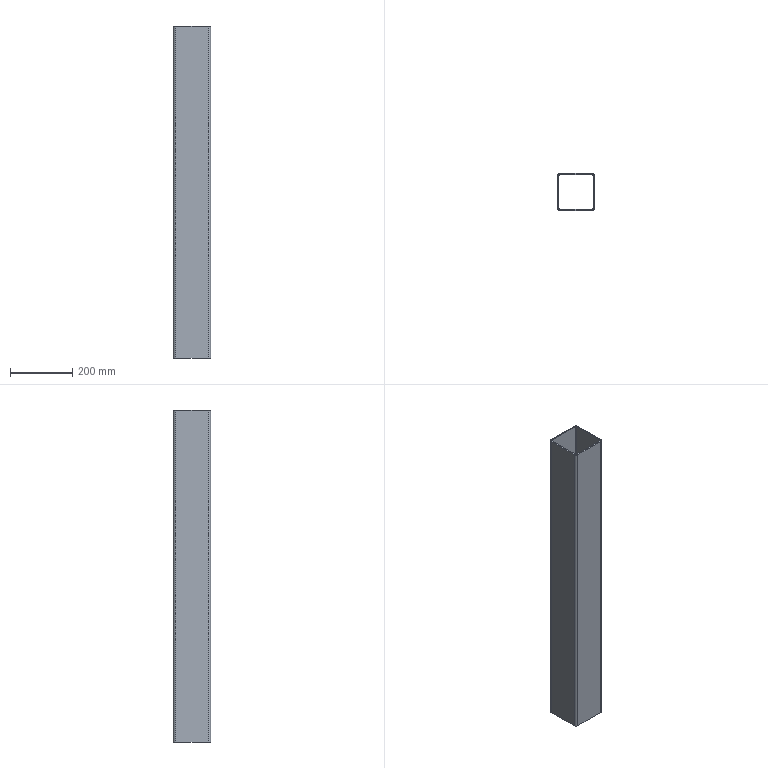Part | SolidWorks | features ICE 1, LibraryFeature 1 | 1 solid | 18 faces | box 120 x 120 x 1070 mm | volume 1941832 mm3 | plane 10 | cylinder 8 | commonest cylinder face diameters 8 x4 16 x4
STEP:
#1=CARTESIAN_POINT('',(52.,60.,-535.));
#2=VERTEX_POINT('',#1);
#3=CARTESIAN_POINT('',(-52.,60.,-535.));
#4=VERTEX_POINT('',#3);
#5=CARTESIAN_POINT('',(0.,60.,-535.));
#6=DIRECTION('',(-1.,0.,0.));
#7=VECTOR('',#6,1000.);
#8=LINE('',#5,#7);
#9=EDGE_CURVE('',#2,#4,#8,.T.);
#10=ORIENTED_EDGE('',*,*,#9,.T.);
#11=CARTESIAN_POINT('',(-52.,60.,535.));
#12=VERTEX_POINT('',#11);
#13=CARTESIAN_POINT('',(-52.,60.,535.));
#14=DIRECTION('',(0.,0.,-1.));
#15=VECTOR('',#14,1000.);
#16=LINE('',#13,#15);
#17=EDGE_CURVE('',#12,#4,#16,.T.);
#18=ORIENTED_EDGE('',*,*,#17,.F.);
#19=CARTESIAN_POINT('',(52.,60.,535.));
#20=VERTEX_POINT('',#19);
#21=CARTESIAN_POINT('',(0.,60.,535.));
#22=DIRECTION('',(-1.,0.,0.));
#23=VECTOR('',#22,1000.);
#24=LINE('',#21,#23);
#25=EDGE_CURVE('',#20,#12,#24,.T.);
#26=ORIENTED_EDGE('',*,*,#25,.F.);
#27=CARTESIAN_POINT('',(52.,60.,535.));
#28=DIRECTION('',(0.,0.,-1.));
#29=VECTOR('',#28,1000.);
#30=LINE('',#27,#29);
#31=EDGE_CURVE('',#20,#2,#30,.T.);
#32=ORIENTED_EDGE('',*,*,#31,.T.);
#33=EDGE_LOOP('',(#10,#18,#26,#32));
#34=FACE_OUTER_BOUND('',#33,.T.);
#35=CARTESIAN_POINT('',(0.,60.,535.));
#36=DIRECTION('',(0.,-1.,0.));
#37=DIRECTION('',(0.,0.,-1.));
#38=AXIS2_PLACEMENT_3D('',#35,#36,#37);
#39=PLANE('',#38);
#40=ADVANCED_FACE('',(#34),#39,.F.);
#41=CARTESIAN_POINT('',(-60.,52.,-535.));
#42=VERTEX_POINT('',#41);
#43=CARTESIAN_POINT('',(-52.,52.,-535.));
#44=DIRECTION('',(0.,0.,1.));
#45=DIRECTION('',(1.,0.,0.));
#46=AXIS2_PLACEMENT_3D('',#43,#44,#45);
#47=CIRCLE('',#46,8.);
#48=EDGE_CURVE('',#4,#42,#47,.T.);
#49=ORIENTED_EDGE('',*,*,#48,.T.);
#50=CARTESIAN_POINT('',(-60.,52.,535.));
#51=VERTEX_POINT('',#50);
#52=CARTESIAN_POINT('',(-60.,52.,535.));
#53=DIRECTION('',(0.,0.,-1.));
#54=VECTOR('',#53,1000.);
#55=LINE('',#52,#54);
#56=EDGE_CURVE('',#51,#42,#55,.T.);
#57=ORIENTED_EDGE('',*,*,#56,.F.);
#58=CARTESIAN_POINT('',(-52.,52.,535.));
#59=DIRECTION('',(0.,0.,1.));
#60=DIRECTION('',(1.,0.,0.));
#61=AXIS2_PLACEMENT_3D('',#58,#59,#60);
#62=CIRCLE('',#61,8.);
#63=EDGE_CURVE('',#12,#51,#62,.T.);
#64=ORIENTED_EDGE('',*,*,#63,.F.);
#65=ORIENTED_EDGE('',*,*,#17,.T.);
#66=EDGE_LOOP('',(#49,#57,#64,#65));
#67=FACE_OUTER_BOUND('',#66,.T.);
#68=CARTESIAN_POINT('',(-52.,52.,535.));
#69=DIRECTION('',(0.,0.,-1.));
#70=DIRECTION('',(-1.,0.,0.));
#71=AXIS2_PLACEMENT_3D('',#68,#69,#70);
#72=CYLINDRICAL_SURFACE('',#71,8.);
#73=ADVANCED_FACE('',(#67),#72,.T.);
#74=CARTESIAN_POINT('',(-60.,-52.,-535.));
#75=VERTEX_POINT('',#74);
#76=CARTESIAN_POINT('',(-60.,0.,-535.));
#77=DIRECTION('',(0.,1.,0.));
#78=VECTOR('',#77,1000.);
#79=LINE('',#76,#78);
#80=EDGE_CURVE('',#75,#42,#79,.T.);
#81=ORIENTED_EDGE('',*,*,#80,.F.);
#82=CARTESIAN_POINT('',(-60.,-52.,535.));
#83=VERTEX_POINT('',#82);
#84=CARTESIAN_POINT('',(-60.,-52.,535.));
#85=DIRECTION('',(0.,0.,-1.));
#86=VECTOR('',#85,1000.);
#87=LINE('',#84,#86);
#88=EDGE_CURVE('',#83,#75,#87,.T.);
#89=ORIENTED_EDGE('',*,*,#88,.F.);
#90=CARTESIAN_POINT('',(-60.,0.,535.));
#91=DIRECTION('',(0.,1.,0.));
#92=VECTOR('',#91,1000.);
#93=LINE('',#90,#92);
#94=EDGE_CURVE('',#83,#51,#93,.T.);
#95=ORIENTED_EDGE('',*,*,#94,.T.);
#96=ORIENTED_EDGE('',*,*,#56,.T.);
#97=EDGE_LOOP('',(#81,#89,#95,#96));
#98=FACE_OUTER_BOUND('',#97,.T.);
#99=CARTESIAN_POINT('',(-60.,0.,535.));
#100=DIRECTION('',(-1.,0.,0.));
#101=DIRECTION('',(0.,0.,1.));
#102=AXIS2_PLACEMENT_3D('',#99,#100,#101);
#103=PLANE('',#102);
#104=ADVANCED_FACE('',(#98),#103,.T.);
#105=CARTESIAN_POINT('',(-52.,-60.,-535.));
#106=VERTEX_POINT('',#105);
#107=CARTESIAN_POINT('',(-52.,-52.,-535.));
#108=DIRECTION('',(0.,0.,1.));
#109=DIRECTION('',(1.,0.,0.));
#110=AXIS2_PLACEMENT_3D('',#107,#108,#109);
#111=CIRCLE('',#110,8.);
#112=EDGE_CURVE('',#75,#106,#111,.T.);
#113=ORIENTED_EDGE('',*,*,#112,.T.);
#114=CARTESIAN_POINT('',(-52.,-60.,535.));
#115=VERTEX_POINT('',#114);
#116=CARTESIAN_POINT('',(-52.,-60.,535.));
#117=DIRECTION('',(0.,0.,-1.));
#118=VECTOR('',#117,1000.);
#119=LINE('',#116,#118);
#120=EDGE_CURVE('',#115,#106,#119,.T.);
#121=ORIENTED_EDGE('',*,*,#120,.F.);
#122=CARTESIAN_POINT('',(-52.,-52.,535.));
#123=DIRECTION('',(0.,0.,1.));
#124=DIRECTION('',(1.,0.,0.));
#125=AXIS2_PLACEMENT_3D('',#122,#123,#124);
#126=CIRCLE('',#125,8.);
#127=EDGE_CURVE('',#83,#115,#126,.T.);
#128=ORIENTED_EDGE('',*,*,#127,.F.);
#129=ORIENTED_EDGE('',*,*,#88,.T.);
#130=EDGE_LOOP('',(#113,#121,#128,#129));
#131=FACE_OUTER_BOUND('',#130,.T.);
#132=CARTESIAN_POINT('',(-52.,-52.,535.));
#133=DIRECTION('',(0.,0.,-1.));
#134=DIRECTION('',(-1.,0.,0.));
#135=AXIS2_PLACEMENT_3D('',#132,#133,#134);
#136=CYLINDRICAL_SURFACE('',#135,8.);
#137=ADVANCED_FACE('',(#131),#136,.T.);
#138=CARTESIAN_POINT('',(52.,-60.,-535.));
#139=VERTEX_POINT('',#138);
#140=CARTESIAN_POINT('',(0.,-60.,-535.));
#141=DIRECTION('',(1.,0.,0.));
#142=VECTOR('',#141,1000.);
#143=LINE('',#140,#142);
#144=EDGE_CURVE('',#106,#139,#143,.T.);
#145=ORIENTED_EDGE('',*,*,#144,.T.);
#146=CARTESIAN_POINT('',(52.,-60.,535.));
#147=VERTEX_POINT('',#146);
#148=CARTESIAN_POINT('',(52.,-60.,535.));
#149=DIRECTION('',(0.,0.,-1.));
#150=VECTOR('',#149,1000.);
#151=LINE('',#148,#150);
#152=EDGE_CURVE('',#147,#139,#151,.T.);
#153=ORIENTED_EDGE('',*,*,#152,.F.);
#154=CARTESIAN_POINT('',(0.,-60.,535.));
#155=DIRECTION('',(1.,0.,0.));
#156=VECTOR('',#155,1000.);
#157=LINE('',#154,#156);
#158=EDGE_CURVE('',#115,#147,#157,.T.);
#159=ORIENTED_EDGE('',*,*,#158,.F.);
#160=ORIENTED_EDGE('',*,*,#120,.T.);
#161=EDGE_LOOP('',(#145,#153,#159,#160));
#162=FACE_OUTER_BOUND('',#161,.T.);
#163=CARTESIAN_POINT('',(0.,-60.,535.));
#164=DIRECTION('',(0.,1.,0.));
#165=DIRECTION('',(0.,0.,1.));
#166=AXIS2_PLACEMENT_3D('',#163,#164,#165);
#167=PLANE('',#166);
#168=ADVANCED_FACE('',(#162),#167,.F.);
#169=CARTESIAN_POINT('',(60.,-52.,-535.));
#170=VERTEX_POINT('',#169);
#171=CARTESIAN_POINT('',(52.,-52.,-535.));
#172=DIRECTION('',(0.,0.,1.));
#173=DIRECTION('',(1.,0.,0.));
#174=AXIS2_PLACEMENT_3D('',#171,#172,#173);
#175=CIRCLE('',#174,8.);
#176=EDGE_CURVE('',#139,#170,#175,.T.);
#177=ORIENTED_EDGE('',*,*,#176,.T.);
#178=CARTESIAN_POINT('',(60.,-52.,535.));
#179=VERTEX_POINT('',#178);
#180=CARTESIAN_POINT('',(60.,-52.,535.));
#181=DIRECTION('',(0.,0.,-1.));
#182=VECTOR('',#181,1000.);
#183=LINE('',#180,#182);
#184=EDGE_CURVE('',#179,#170,#183,.T.);
#185=ORIENTED_EDGE('',*,*,#184,.F.);
#186=CARTESIAN_POINT('',(52.,-52.,535.));
#187=DIRECTION('',(0.,0.,1.));
#188=DIRECTION('',(1.,0.,0.));
#189=AXIS2_PLACEMENT_3D('',#186,#187,#188);
#190=CIRCLE('',#189,8.);
#191=EDGE_CURVE('',#147,#179,#190,.T.);
#192=ORIENTED_EDGE('',*,*,#191,.F.);
#193=ORIENTED_EDGE('',*,*,#152,.T.);
#194=EDGE_LOOP('',(#177,#185,#192,#193));
#195=FACE_OUTER_BOUND('',#194,.T.);
#196=CARTESIAN_POINT('',(52.,-52.,535.));
#197=DIRECTION('',(0.,0.,-1.));
#198=DIRECTION('',(-1.,0.,0.));
#199=AXIS2_PLACEMENT_3D('',#196,#197,#198);
#200=CYLINDRICAL_SURFACE('',#199,8.);
#201=ADVANCED_FACE('',(#195),#200,.T.);
#202=CARTESIAN_POINT('',(60.,52.,-535.));
#203=VERTEX_POINT('',#202);
#204=CARTESIAN_POINT('',(60.,0.,-535.));
#205=DIRECTION('',(0.,-1.,0.));
#206=VECTOR('',#205,1000.);
#207=LINE('',#204,#206);
#208=EDGE_CURVE('',#203,#170,#207,.T.);
#209=ORIENTED_EDGE('',*,*,#208,.F.);
#210=CARTESIAN_POINT('',(60.,52.,535.));
#211=VERTEX_POINT('',#210);
#212=CARTESIAN_POINT('',(60.,52.,535.));
#213=DIRECTION('',(0.,0.,-1.));
#214=VECTOR('',#213,1000.);
#215=LINE('',#212,#214);
#216=EDGE_CURVE('',#211,#203,#215,.T.);
#217=ORIENTED_EDGE('',*,*,#216,.F.);
#218=CARTESIAN_POINT('',(60.,0.,535.));
#219=DIRECTION('',(0.,-1.,0.));
#220=VECTOR('',#219,1000.);
#221=LINE('',#218,#220);
#222=EDGE_CURVE('',#211,#179,#221,.T.);
#223=ORIENTED_EDGE('',*,*,#222,.T.);
#224=ORIENTED_EDGE('',*,*,#184,.T.);
#225=EDGE_LOOP('',(#209,#217,#223,#224));
#226=FACE_OUTER_BOUND('',#225,.T.);
#227=CARTESIAN_POINT('',(60.,0.,535.));
#228=DIRECTION('',(1.,0.,0.));
#229=DIRECTION('',(0.,0.,-1.));
#230=AXIS2_PLACEMENT_3D('',#227,#228,#229);
#231=PLANE('',#230);
#232=ADVANCED_FACE('',(#226),#231,.T.);
#233=CARTESIAN_POINT('',(-56.,-52.,-535.));
#234=VERTEX_POINT('',#233);
#235=CARTESIAN_POINT('',(-52.,-56.,-535.));
#236=VERTEX_POINT('',#235);
#237=CARTESIAN_POINT('',(-52.,-52.,-535.));
#238=DIRECTION('',(0.,0.,1.));
#239=DIRECTION('',(1.,0.,0.));
#240=AXIS2_PLACEMENT_3D('',#237,#238,#239);
#241=CIRCLE('',#240,4.);
#242=EDGE_CURVE('',#234,#236,#241,.T.);
#243=ORIENTED_EDGE('',*,*,#242,.F.);
#244=CARTESIAN_POINT('',(-56.,-52.,535.));
#245=VERTEX_POINT('',#244);
#246=CARTESIAN_POINT('',(-56.,-52.,535.));
#247=DIRECTION('',(0.,0.,-1.));
#248=VECTOR('',#247,1000.);
#249=LINE('',#246,#248);
#250=EDGE_CURVE('',#245,#234,#249,.T.);
#251=ORIENTED_EDGE('',*,*,#250,.F.);
#252=CARTESIAN_POINT('',(-52.,-56.,535.));
#253=VERTEX_POINT('',#252);
#254=CARTESIAN_POINT('',(-52.,-52.,535.));
#255=DIRECTION('',(0.,0.,1.));
#256=DIRECTION('',(1.,0.,0.));
#257=AXIS2_PLACEMENT_3D('',#254,#255,#256);
#258=CIRCLE('',#257,4.);
#259=EDGE_CURVE('',#245,#253,#258,.T.);
#260=ORIENTED_EDGE('',*,*,#259,.T.);
#261=CARTESIAN_POINT('',(-52.,-56.,535.));
#262=DIRECTION('',(0.,0.,-1.));
#263=VECTOR('',#262,1000.);
#264=LINE('',#261,#263);
#265=EDGE_CURVE('',#253,#236,#264,.T.);
#266=ORIENTED_EDGE('',*,*,#265,.T.);
#267=EDGE_LOOP('',(#243,#251,#260,#266));
#268=FACE_OUTER_BOUND('',#267,.T.);
#269=CARTESIAN_POINT('',(-52.,-52.,535.));
#270=DIRECTION('',(0.,0.,-1.));
#271=DIRECTION('',(-1.,0.,0.));
#272=AXIS2_PLACEMENT_3D('',#269,#270,#271);
#273=CYLINDRICAL_SURFACE('',#272,4.);
#274=ADVANCED_FACE('',(#268),#273,.F.);
#275=CARTESIAN_POINT('',(-56.,52.,-535.));
#276=VERTEX_POINT('',#275);
#277=CARTESIAN_POINT('',(-56.,0.,-535.));
#278=DIRECTION('',(0.,1.,0.));
#279=VECTOR('',#278,1000.);
#280=LINE('',#277,#279);
#281=EDGE_CURVE('',#234,#276,#280,.T.);
#282=ORIENTED_EDGE('',*,*,#281,.T.);
#283=CARTESIAN_POINT('',(-56.,52.,535.));
#284=VERTEX_POINT('',#283);
#285=CARTESIAN_POINT('',(-56.,52.,535.));
#286=DIRECTION('',(0.,0.,-1.));
#287=VECTOR('',#286,1000.);
#288=LINE('',#285,#287);
#289=EDGE_CURVE('',#284,#276,#288,.T.);
#290=ORIENTED_EDGE('',*,*,#289,.F.);
#291=CARTESIAN_POINT('',(-56.,0.,535.));
#292=DIRECTION('',(0.,1.,0.));
#293=VECTOR('',#292,1000.);
#294=LINE('',#291,#293);
#295=EDGE_CURVE('',#245,#284,#294,.T.);
#296=ORIENTED_EDGE('',*,*,#295,.F.);
#297=ORIENTED_EDGE('',*,*,#250,.T.);
#298=EDGE_LOOP('',(#282,#290,#296,#297));
#299=FACE_OUTER_BOUND('',#298,.T.);
#300=CARTESIAN_POINT('',(-56.,0.,535.));
#301=DIRECTION('',(-1.,0.,0.));
#302=DIRECTION('',(0.,0.,1.));
#303=AXIS2_PLACEMENT_3D('',#300,#301,#302);
#304=PLANE('',#303);
#305=ADVANCED_FACE('',(#299),#304,.F.);
#306=CARTESIAN_POINT('',(-52.,56.,-535.));
#307=VERTEX_POINT('',#306);
#308=CARTESIAN_POINT('',(-52.,52.,-535.));
#309=DIRECTION('',(0.,0.,1.));
#310=DIRECTION('',(1.,0.,0.));
#311=AXIS2_PLACEMENT_3D('',#308,#309,#310);
#312=CIRCLE('',#311,4.);
#313=EDGE_CURVE('',#307,#276,#312,.T.);
#314=ORIENTED_EDGE('',*,*,#313,.F.);
#315=CARTESIAN_POINT('',(-52.,56.,535.));
#316=VERTEX_POINT('',#315);
#317=CARTESIAN_POINT('',(-52.,56.,535.));
#318=DIRECTION('',(0.,0.,-1.));
#319=VECTOR('',#318,1000.);
#320=LINE('',#317,#319);
#321=EDGE_CURVE('',#316,#307,#320,.T.);
#322=ORIENTED_EDGE('',*,*,#321,.F.);
#323=CARTESIAN_POINT('',(-52.,52.,535.));
#324=DIRECTION('',(0.,0.,1.));
#325=DIRECTION('',(1.,0.,0.));
#326=AXIS2_PLACEMENT_3D('',#323,#324,#325);
#327=CIRCLE('',#326,4.);
#328=EDGE_CURVE('',#316,#284,#327,.T.);
#329=ORIENTED_EDGE('',*,*,#328,.T.);
#330=ORIENTED_EDGE('',*,*,#289,.T.);
#331=EDGE_LOOP('',(#314,#322,#329,#330));
#332=FACE_OUTER_BOUND('',#331,.T.);
#333=CARTESIAN_POINT('',(-52.,52.,535.));
#334=DIRECTION('',(0.,0.,-1.));
#335=DIRECTION('',(-1.,0.,0.));
#336=AXIS2_PLACEMENT_3D('',#333,#334,#335);
#337=CYLINDRICAL_SURFACE('',#336,4.);
#338=ADVANCED_FACE('',(#332),#337,.F.);
#339=CARTESIAN_POINT('',(52.,56.,-535.));
#340=VERTEX_POINT('',#339);
#341=CARTESIAN_POINT('',(0.,56.,-535.));
#342=DIRECTION('',(-1.,0.,0.));
#343=VECTOR('',#342,1000.);
#344=LINE('',#341,#343);
#345=EDGE_CURVE('',#340,#307,#344,.T.);
#346=ORIENTED_EDGE('',*,*,#345,.F.);
#347=CARTESIAN_POINT('',(52.,56.,535.));
#348=VERTEX_POINT('',#347);
#349=CARTESIAN_POINT('',(52.,56.,535.));
#350=DIRECTION('',(0.,0.,-1.));
#351=VECTOR('',#350,1000.);
#352=LINE('',#349,#351);
#353=EDGE_CURVE('',#348,#340,#352,.T.);
#354=ORIENTED_EDGE('',*,*,#353,.F.);
#355=CARTESIAN_POINT('',(0.,56.,535.));
#356=DIRECTION('',(-1.,0.,0.));
#357=VECTOR('',#356,1000.);
#358=LINE('',#355,#357);
#359=EDGE_CURVE('',#348,#316,#358,.T.);
#360=ORIENTED_EDGE('',*,*,#359,.T.);
#361=ORIENTED_EDGE('',*,*,#321,.T.);
#362=EDGE_LOOP('',(#346,#354,#360,#361));
#363=FACE_OUTER_BOUND('',#362,.T.);
#364=CARTESIAN_POINT('',(0.,56.,535.));
#365=DIRECTION('',(0.,-1.,0.));
#366=DIRECTION('',(0.,0.,-1.));
#367=AXIS2_PLACEMENT_3D('',#364,#365,#366);
#368=PLANE('',#367);
#369=ADVANCED_FACE('',(#363),#368,.T.);
#370=CARTESIAN_POINT('',(56.,52.,-535.));
#371=VERTEX_POINT('',#370);
#372=CARTESIAN_POINT('',(52.,52.,-535.));
#373=DIRECTION('',(0.,0.,1.));
#374=DIRECTION('',(1.,0.,0.));
#375=AXIS2_PLACEMENT_3D('',#372,#373,#374);
#376=CIRCLE('',#375,4.);
#377=EDGE_CURVE('',#371,#340,#376,.T.);
#378=ORIENTED_EDGE('',*,*,#377,.F.);
#379=CARTESIAN_POINT('',(56.,52.,535.));
#380=VERTEX_POINT('',#379);
#381=CARTESIAN_POINT('',(56.,52.,535.));
#382=DIRECTION('',(0.,0.,-1.));
#383=VECTOR('',#382,1000.);
#384=LINE('',#381,#383);
#385=EDGE_CURVE('',#380,#371,#384,.T.);
#386=ORIENTED_EDGE('',*,*,#385,.F.);
#387=CARTESIAN_POINT('',(52.,52.,535.));
#388=DIRECTION('',(0.,0.,1.));
#389=DIRECTION('',(1.,0.,0.));
#390=AXIS2_PLACEMENT_3D('',#387,#388,#389);
#391=CIRCLE('',#390,4.);
#392=EDGE_CURVE('',#380,#348,#391,.T.);
#393=ORIENTED_EDGE('',*,*,#392,.T.);
#394=ORIENTED_EDGE('',*,*,#353,.T.);
#395=EDGE_LOOP('',(#378,#386,#393,#394));
#396=FACE_OUTER_BOUND('',#395,.T.);
#397=CARTESIAN_POINT('',(52.,52.,535.));
#398=DIRECTION('',(0.,0.,-1.));
#399=DIRECTION('',(-1.,0.,0.));
#400=AXIS2_PLACEMENT_3D('',#397,#398,#399);
#401=CYLINDRICAL_SURFACE('',#400,4.);
#402=ADVANCED_FACE('',(#396),#401,.F.);
#403=CARTESIAN_POINT('',(56.,-52.,-535.));
#404=VERTEX_POINT('',#403);
#405=CARTESIAN_POINT('',(56.,0.,-535.));
#406=DIRECTION('',(0.,-1.,0.));
#407=VECTOR('',#406,1000.);
#408=LINE('',#405,#407);
#409=EDGE_CURVE('',#371,#404,#408,.T.);
#410=ORIENTED_EDGE('',*,*,#409,.T.);
#411=CARTESIAN_POINT('',(56.,-52.,535.));
#412=VERTEX_POINT('',#411);
#413=CARTESIAN_POINT('',(56.,-52.,535.));
#414=DIRECTION('',(0.,0.,-1.));
#415=VECTOR('',#414,1000.);
#416=LINE('',#413,#415);
#417=EDGE_CURVE('',#412,#404,#416,.T.);
#418=ORIENTED_EDGE('',*,*,#417,.F.);
#419=CARTESIAN_POINT('',(56.,0.,535.));
#420=DIRECTION('',(0.,-1.,0.));
#421=VECTOR('',#420,1000.);
#422=LINE('',#419,#421);
#423=EDGE_CURVE('',#380,#412,#422,.T.);
#424=ORIENTED_EDGE('',*,*,#423,.F.);
#425=ORIENTED_EDGE('',*,*,#385,.T.);
#426=EDGE_LOOP('',(#410,#418,#424,#425));
#427=FACE_OUTER_BOUND('',#426,.T.);
#428=CARTESIAN_POINT('',(56.,0.,535.));
#429=DIRECTION('',(1.,0.,0.));
#430=DIRECTION('',(0.,0.,-1.));
#431=AXIS2_PLACEMENT_3D('',#428,#429,#430);
#432=PLANE('',#431);
#433=ADVANCED_FACE('',(#427),#432,.F.);
#434=CARTESIAN_POINT('',(52.,-56.,-535.));
#435=VERTEX_POINT('',#434);
#436=CARTESIAN_POINT('',(52.,-52.,-535.));
#437=DIRECTION('',(0.,0.,1.));
#438=DIRECTION('',(1.,0.,0.));
#439=AXIS2_PLACEMENT_3D('',#436,#437,#438);
#440=CIRCLE('',#439,4.);
#441=EDGE_CURVE('',#435,#404,#440,.T.);
#442=ORIENTED_EDGE('',*,*,#441,.F.);
#443=CARTESIAN_POINT('',(52.,-56.,535.));
#444=VERTEX_POINT('',#443);
#445=CARTESIAN_POINT('',(52.,-56.,535.));
#446=DIRECTION('',(0.,0.,-1.));
#447=VECTOR('',#446,1000.);
#448=LINE('',#445,#447);
#449=EDGE_CURVE('',#444,#435,#448,.T.);
#450=ORIENTED_EDGE('',*,*,#449,.F.);
#451=CARTESIAN_POINT('',(52.,-52.,535.));
#452=DIRECTION('',(0.,0.,1.));
#453=DIRECTION('',(1.,0.,0.));
#454=AXIS2_PLACEMENT_3D('',#451,#452,#453);
#455=CIRCLE('',#454,4.);
#456=EDGE_CURVE('',#444,#412,#455,.T.);
#457=ORIENTED_EDGE('',*,*,#456,.T.);
#458=ORIENTED_EDGE('',*,*,#417,.T.);
#459=EDGE_LOOP('',(#442,#450,#457,#458));
#460=FACE_OUTER_BOUND('',#459,.T.);
#461=CARTESIAN_POINT('',(52.,-52.,535.));
#462=DIRECTION('',(0.,0.,-1.));
#463=DIRECTION('',(-1.,0.,0.));
#464=AXIS2_PLACEMENT_3D('',#461,#462,#463);
#465=CYLINDRICAL_SURFACE('',#464,4.);
#466=ADVANCED_FACE('',(#460),#465,.F.);
#467=CARTESIAN_POINT('',(0.,-56.,-535.));
#468=DIRECTION('',(1.,0.,0.));
#469=VECTOR('',#468,1000.);
#470=LINE('',#467,#469);
#471=EDGE_CURVE('',#236,#435,#470,.T.);
#472=ORIENTED_EDGE('',*,*,#471,.F.);
#473=ORIENTED_EDGE('',*,*,#265,.F.);
#474=CARTESIAN_POINT('',(0.,-56.,535.));
#475=DIRECTION('',(1.,0.,0.));
#476=VECTOR('',#475,1000.);
#477=LINE('',#474,#476);
#478=EDGE_CURVE('',#253,#444,#477,.T.);
#479=ORIENTED_EDGE('',*,*,#478,.T.);
#480=ORIENTED_EDGE('',*,*,#449,.T.);
#481=EDGE_LOOP('',(#472,#473,#479,#480));
#482=FACE_OUTER_BOUND('',#481,.T.);
#483=CARTESIAN_POINT('',(0.,-56.,535.));
#484=DIRECTION('',(0.,1.,0.));
#485=DIRECTION('',(0.,0.,1.));
#486=AXIS2_PLACEMENT_3D('',#483,#484,#485);
#487=PLANE('',#486);
#488=ADVANCED_FACE('',(#482),#487,.T.);
#489=CARTESIAN_POINT('',(52.,52.,-535.));
#490=DIRECTION('',(0.,0.,1.));
#491=DIRECTION('',(1.,0.,0.));
#492=AXIS2_PLACEMENT_3D('',#489,#490,#491);
#493=CIRCLE('',#492,8.);
#494=EDGE_CURVE('',#203,#2,#493,.T.);
#495=ORIENTED_EDGE('',*,*,#494,.T.);
#496=ORIENTED_EDGE('',*,*,#31,.F.);
#497=CARTESIAN_POINT('',(52.,52.,535.));
#498=DIRECTION('',(0.,0.,1.));
#499=DIRECTION('',(1.,0.,0.));
#500=AXIS2_PLACEMENT_3D('',#497,#498,#499);
#501=CIRCLE('',#500,8.);
#502=EDGE_CURVE('',#211,#20,#501,.T.);
#503=ORIENTED_EDGE('',*,*,#502,.F.);
#504=ORIENTED_EDGE('',*,*,#216,.T.);
#505=EDGE_LOOP('',(#495,#496,#503,#504));
#506=FACE_OUTER_BOUND('',#505,.T.);
#507=CARTESIAN_POINT('',(52.,52.,535.));
#508=DIRECTION('',(0.,0.,-1.));
#509=DIRECTION('',(-1.,0.,0.));
#510=AXIS2_PLACEMENT_3D('',#507,#508,#509);
#511=CYLINDRICAL_SURFACE('',#510,8.);
#512=ADVANCED_FACE('',(#506),#511,.T.);
#513=ORIENTED_EDGE('',*,*,#259,.F.);
#514=ORIENTED_EDGE('',*,*,#295,.T.);
#515=ORIENTED_EDGE('',*,*,#328,.F.);
#516=ORIENTED_EDGE('',*,*,#359,.F.);
#517=ORIENTED_EDGE('',*,*,#392,.F.);
#518=ORIENTED_EDGE('',*,*,#423,.T.);
#519=ORIENTED_EDGE('',*,*,#456,.F.);
#520=ORIENTED_EDGE('',*,*,#478,.F.);
#521=EDGE_LOOP('',(#513,#514,#515,#516,#517,#518,#519,#520));
#522=FACE_BOUND('',#521,.T.);
#523=ORIENTED_EDGE('',*,*,#25,.T.);
#524=ORIENTED_EDGE('',*,*,#63,.T.);
#525=ORIENTED_EDGE('',*,*,#94,.F.);
#526=ORIENTED_EDGE('',*,*,#127,.T.);
#527=ORIENTED_EDGE('',*,*,#158,.T.);
#528=ORIENTED_EDGE('',*,*,#191,.T.);
#529=ORIENTED_EDGE('',*,*,#222,.F.);
#530=ORIENTED_EDGE('',*,*,#502,.T.);
#531=EDGE_LOOP('',(#523,#524,#525,#526,#527,#528,#529,#530));
#532=FACE_OUTER_BOUND('',#531,.T.);
#533=CARTESIAN_POINT('',(0.,0.,535.));
#534=DIRECTION('',(0.,0.,1.));
#535=DIRECTION('',(1.,0.,0.));
#536=AXIS2_PLACEMENT_3D('',#533,#534,#535);
#537=PLANE('',#536);
#538=ADVANCED_FACE('',(#522,#532),#537,.T.);
#539=ORIENTED_EDGE('',*,*,#242,.T.);
#540=ORIENTED_EDGE('',*,*,#471,.T.);
#541=ORIENTED_EDGE('',*,*,#441,.T.);
#542=ORIENTED_EDGE('',*,*,#409,.F.);
#543=ORIENTED_EDGE('',*,*,#377,.T.);
#544=ORIENTED_EDGE('',*,*,#345,.T.);
#545=ORIENTED_EDGE('',*,*,#313,.T.);
#546=ORIENTED_EDGE('',*,*,#281,.F.);
#547=EDGE_LOOP('',(#539,#540,#541,#542,#543,#544,#545,#546));
#548=FACE_BOUND('',#547,.T.);
#549=ORIENTED_EDGE('',*,*,#9,.F.);
#550=ORIENTED_EDGE('',*,*,#494,.F.);
#551=ORIENTED_EDGE('',*,*,#208,.T.);
#552=ORIENTED_EDGE('',*,*,#176,.F.);
#553=ORIENTED_EDGE('',*,*,#144,.F.);
#554=ORIENTED_EDGE('',*,*,#112,.F.);
#555=ORIENTED_EDGE('',*,*,#80,.T.);
#556=ORIENTED_EDGE('',*,*,#48,.F.);
#557=EDGE_LOOP('',(#549,#550,#551,#552,#553,#554,#555,#556));
#558=FACE_OUTER_BOUND('',#557,.T.);
#559=CARTESIAN_POINT('',(0.,0.,-535.));
#560=DIRECTION('',(0.,0.,1.));
#561=DIRECTION('',(1.,0.,0.));
#562=AXIS2_PLACEMENT_3D('',#559,#560,#561);
#563=PLANE('',#562);
#564=ADVANCED_FACE('',(#548,#558),#563,.F.);
#565=CLOSED_SHELL('',(#40,#73,#104,#137,#168,#201,#232,#274,#305,#338,#369,#402,#433,#466,#488,#512,#538,#564));
#566=MANIFOLD_SOLID_BREP('',#565);
#567=CARTESIAN_POINT('',(0.,0.,0.));
#568=DIRECTION('',(0.,0.,1.));
#569=DIRECTION('',(1.,0.,0.));
#570=AXIS2_PLACEMENT_3D('',#567,#568,#569);
#571=(LENGTH_UNIT()NAMED_UNIT(*)SI_UNIT(.MILLI.,.METRE.));
#572=UNCERTAINTY_MEASURE_WITH_UNIT(LENGTH_MEASURE(0.00001),#571,'','');
#573=(NAMED_UNIT(*)PLANE_ANGLE_UNIT()SI_UNIT($,.RADIAN.));
#574=(NAMED_UNIT(*)SI_UNIT($,.STERADIAN.)SOLID_ANGLE_UNIT());
#575=(GEOMETRIC_REPRESENTATION_CONTEXT(3)GLOBAL_UNCERTAINTY_ASSIGNED_CONTEXT((#572))GLOBAL_UNIT_ASSIGNED_CONTEXT((#571,#573,#574))REPRESENTATION_CONTEXT('',''));
#576=ADVANCED_BREP_SHAPE_REPRESENTATION('',(#566,#570),#575);